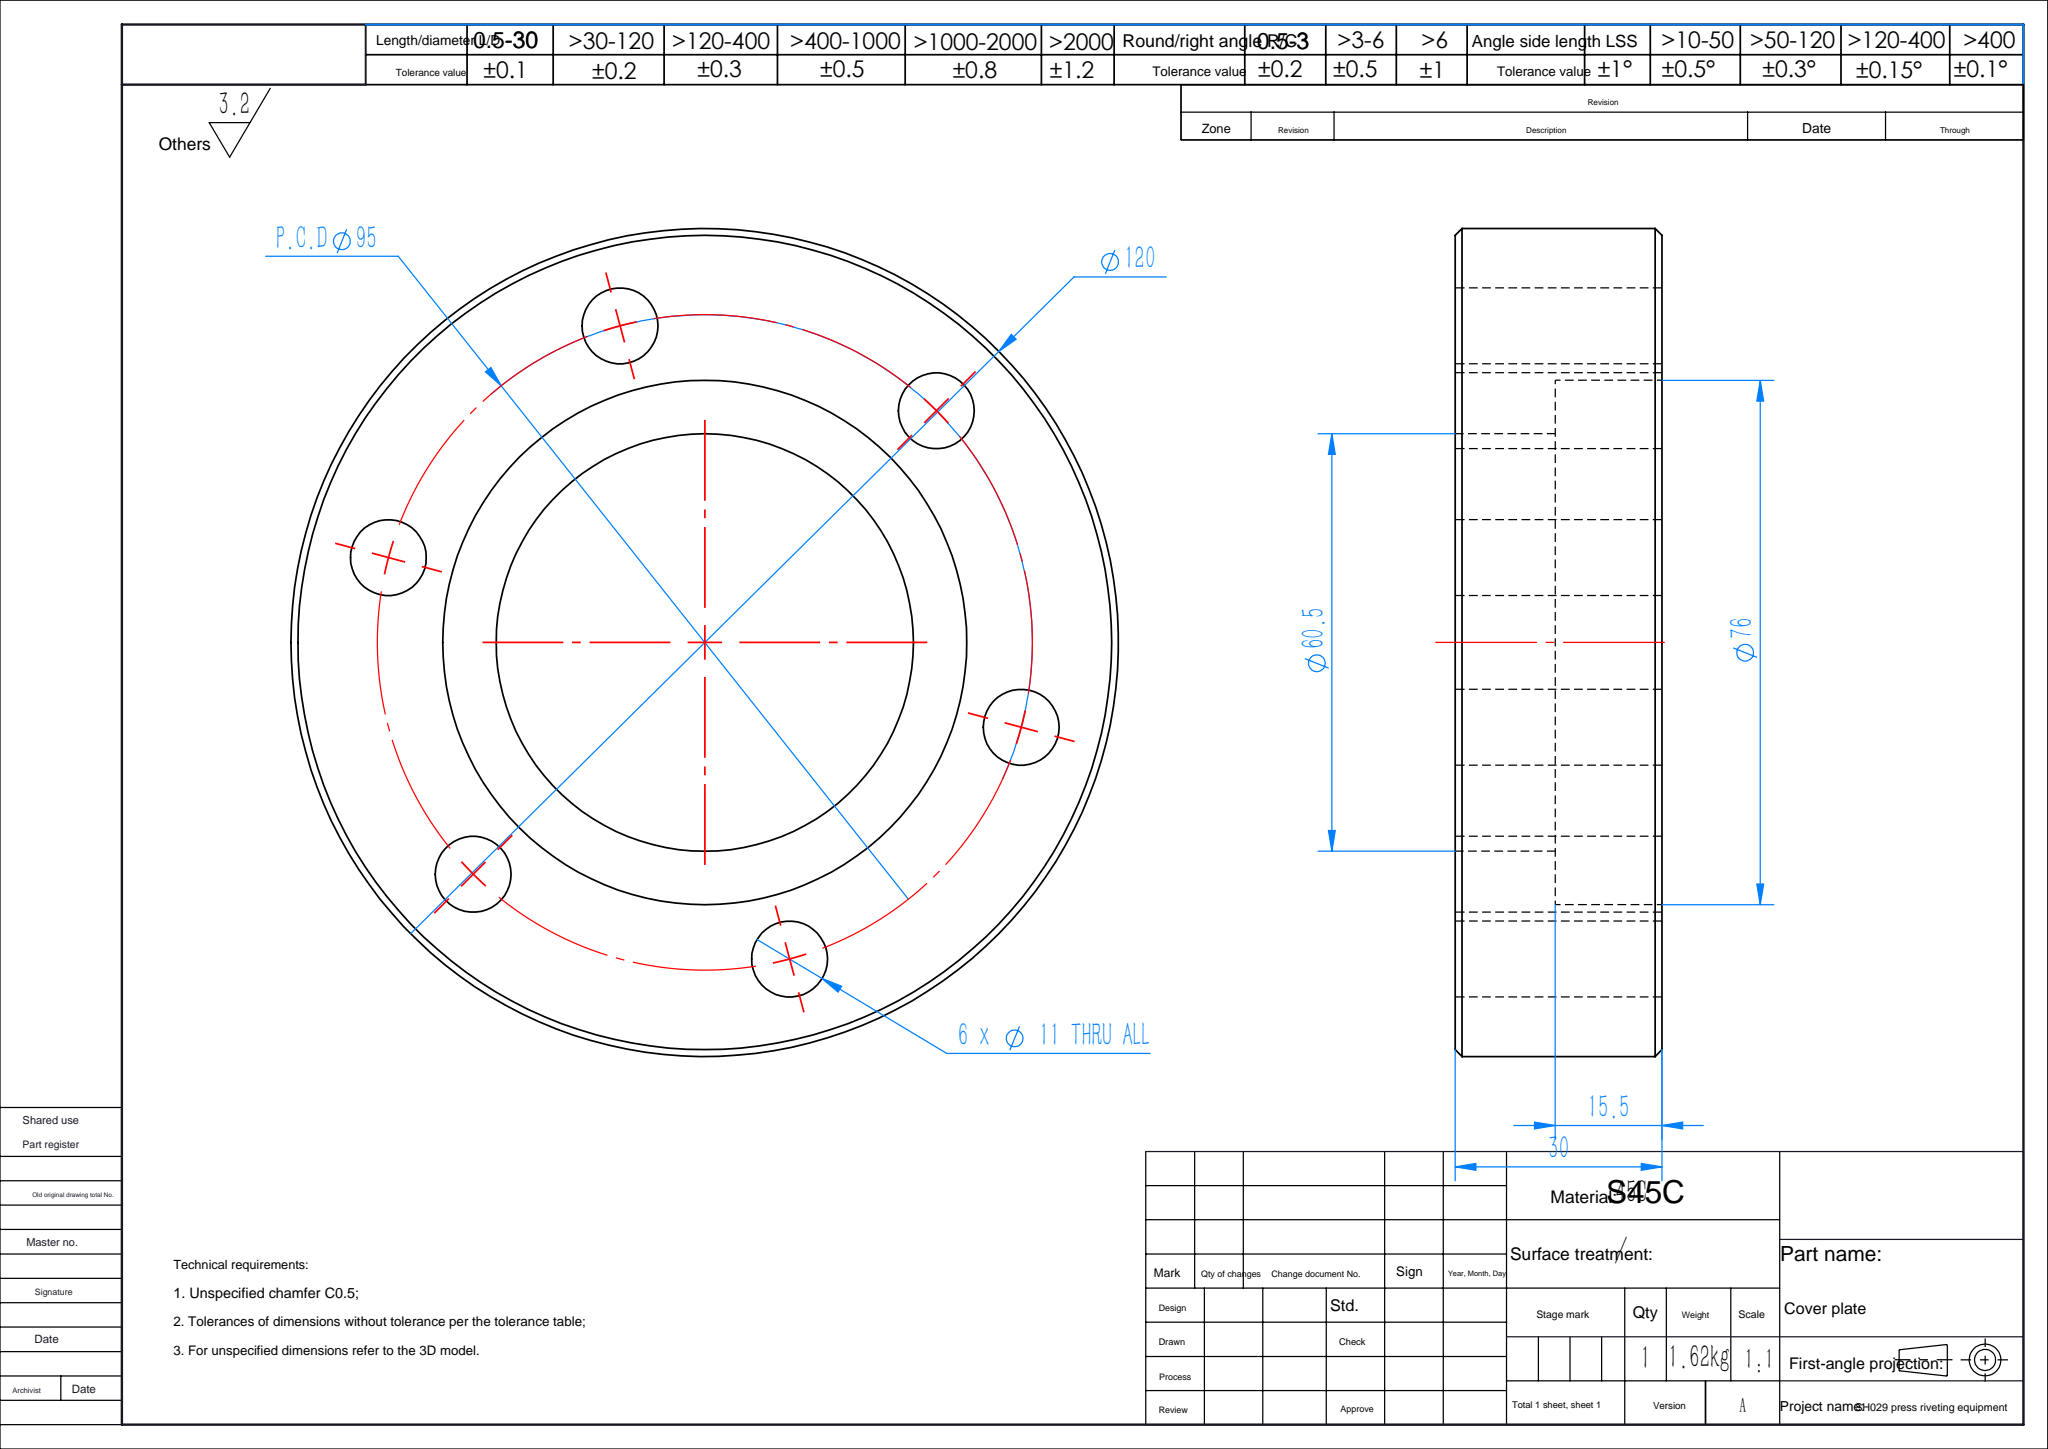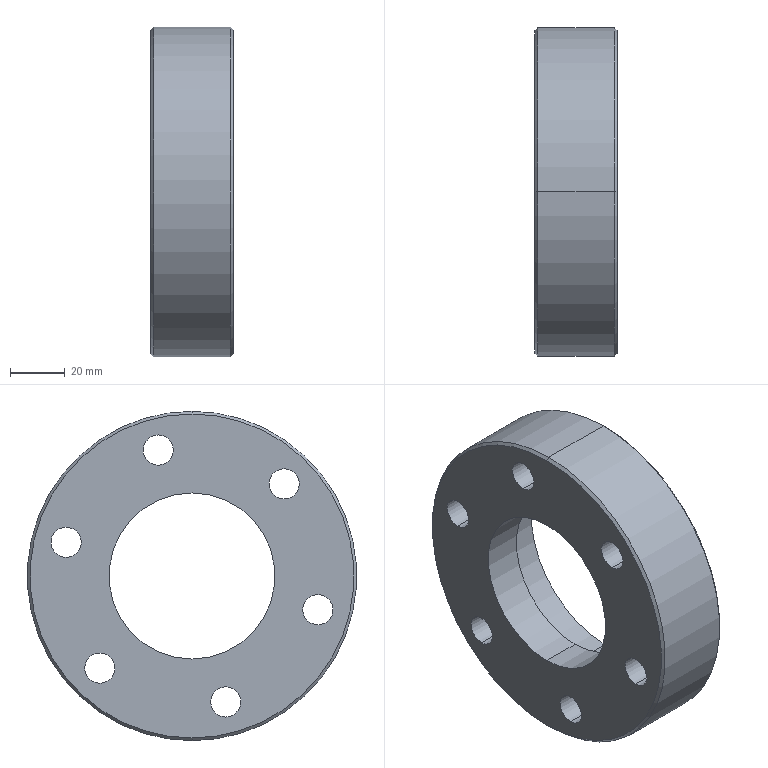Part | SolidWorks | features Chamfer 1, CirPattern 1, HoleWzd 1, Revolution 1 | 1 solid | 25 faces | box 30 x 120 x 120 mm | volume 209812 mm3 | cylinder 18 | cone 4 | plane 3 | commonest cylinder face diameters 11 x12 60.5 x2 76 x2 120 x2
STEP:
#1=CARTESIAN_POINT('',(15.,12.294,40.381));
#2=VERTEX_POINT('',#1);
#3=CARTESIAN_POINT('',(15.,12.294,51.381));
#4=VERTEX_POINT('',#3);
#5=CARTESIAN_POINT('',(15.,12.294,45.881));
#6=DIRECTION('',(-1.,0.,0.));
#7=DIRECTION('',(0.,0.,1.));
#8=AXIS2_PLACEMENT_3D('',#5,#6,#7);
#9=CIRCLE('',#8,5.5);
#10=EDGE_CURVE('',#2,#4,#9,.T.);
#11=ORIENTED_EDGE('',*,*,#10,.F.);
#12=CARTESIAN_POINT('',(-15.,12.294,40.381));
#13=VERTEX_POINT('',#12);
#14=CARTESIAN_POINT('',(-15.,12.294,40.381));
#15=DIRECTION('',(-1.,0.,0.));
#16=VECTOR('',#15,1000.);
#17=LINE('',#14,#16);
#18=EDGE_CURVE('',#2,#13,#17,.T.);
#19=ORIENTED_EDGE('',*,*,#18,.T.);
#20=CARTESIAN_POINT('',(-15.,12.294,51.381));
#21=VERTEX_POINT('',#20);
#22=CARTESIAN_POINT('',(-15.,12.294,45.881));
#23=DIRECTION('',(-1.,0.,0.));
#24=DIRECTION('',(0.,0.,1.));
#25=AXIS2_PLACEMENT_3D('',#22,#23,#24);
#26=CIRCLE('',#25,5.5);
#27=EDGE_CURVE('',#13,#21,#26,.T.);
#28=ORIENTED_EDGE('',*,*,#27,.T.);
#29=CARTESIAN_POINT('',(-15.,12.294,51.381));
#30=DIRECTION('',(-1.,0.,0.));
#31=VECTOR('',#30,1000.);
#32=LINE('',#29,#31);
#33=EDGE_CURVE('',#4,#21,#32,.T.);
#34=ORIENTED_EDGE('',*,*,#33,.F.);
#35=EDGE_LOOP('',(#11,#19,#28,#34));
#36=FACE_OUTER_BOUND('',#35,.T.);
#37=CARTESIAN_POINT('',(-15.,12.294,45.881));
#38=DIRECTION('',(-1.,0.,0.));
#39=DIRECTION('',(0.,0.,1.));
#40=AXIS2_PLACEMENT_3D('',#37,#38,#39);
#41=CYLINDRICAL_SURFACE('',#40,5.5);
#42=ADVANCED_FACE('',(#36),#41,.F.);
#43=CARTESIAN_POINT('',(15.,45.881,6.794));
#44=VERTEX_POINT('',#43);
#45=CARTESIAN_POINT('',(15.,45.881,17.794));
#46=VERTEX_POINT('',#45);
#47=CARTESIAN_POINT('',(15.,45.881,12.294));
#48=DIRECTION('',(-1.,0.,0.));
#49=DIRECTION('',(0.,0.,1.));
#50=AXIS2_PLACEMENT_3D('',#47,#48,#49);
#51=CIRCLE('',#50,5.5);
#52=EDGE_CURVE('',#44,#46,#51,.T.);
#53=ORIENTED_EDGE('',*,*,#52,.F.);
#54=CARTESIAN_POINT('',(-15.,45.881,6.794));
#55=VERTEX_POINT('',#54);
#56=CARTESIAN_POINT('',(-15.,45.881,6.794));
#57=DIRECTION('',(-1.,0.,0.));
#58=VECTOR('',#57,1000.);
#59=LINE('',#56,#58);
#60=EDGE_CURVE('',#44,#55,#59,.T.);
#61=ORIENTED_EDGE('',*,*,#60,.T.);
#62=CARTESIAN_POINT('',(-15.,45.881,17.794));
#63=VERTEX_POINT('',#62);
#64=CARTESIAN_POINT('',(-15.,45.881,12.294));
#65=DIRECTION('',(-1.,0.,0.));
#66=DIRECTION('',(0.,0.,1.));
#67=AXIS2_PLACEMENT_3D('',#64,#65,#66);
#68=CIRCLE('',#67,5.5);
#69=EDGE_CURVE('',#55,#63,#68,.T.);
#70=ORIENTED_EDGE('',*,*,#69,.T.);
#71=CARTESIAN_POINT('',(-15.,45.881,17.794));
#72=DIRECTION('',(-1.,0.,0.));
#73=VECTOR('',#72,1000.);
#74=LINE('',#71,#73);
#75=EDGE_CURVE('',#46,#63,#74,.T.);
#76=ORIENTED_EDGE('',*,*,#75,.F.);
#77=EDGE_LOOP('',(#53,#61,#70,#76));
#78=FACE_OUTER_BOUND('',#77,.T.);
#79=CARTESIAN_POINT('',(-15.,45.881,12.294));
#80=DIRECTION('',(-1.,0.,0.));
#81=DIRECTION('',(0.,0.,1.));
#82=AXIS2_PLACEMENT_3D('',#79,#80,#81);
#83=CYLINDRICAL_SURFACE('',#82,5.5);
#84=ADVANCED_FACE('',(#78),#83,.F.);
#85=CARTESIAN_POINT('',(15.,33.588,-39.088));
#86=VERTEX_POINT('',#85);
#87=CARTESIAN_POINT('',(15.,33.588,-28.088));
#88=VERTEX_POINT('',#87);
#89=CARTESIAN_POINT('',(15.,33.588,-33.588));
#90=DIRECTION('',(-1.,0.,0.));
#91=DIRECTION('',(0.,0.,1.));
#92=AXIS2_PLACEMENT_3D('',#89,#90,#91);
#93=CIRCLE('',#92,5.5);
#94=EDGE_CURVE('',#86,#88,#93,.T.);
#95=ORIENTED_EDGE('',*,*,#94,.F.);
#96=CARTESIAN_POINT('',(-15.,33.588,-39.088));
#97=VERTEX_POINT('',#96);
#98=CARTESIAN_POINT('',(-15.,33.588,-39.088));
#99=DIRECTION('',(-1.,0.,0.));
#100=VECTOR('',#99,1000.);
#101=LINE('',#98,#100);
#102=EDGE_CURVE('',#86,#97,#101,.T.);
#103=ORIENTED_EDGE('',*,*,#102,.T.);
#104=CARTESIAN_POINT('',(-15.,33.588,-28.088));
#105=VERTEX_POINT('',#104);
#106=CARTESIAN_POINT('',(-15.,33.588,-33.588));
#107=DIRECTION('',(-1.,0.,0.));
#108=DIRECTION('',(0.,0.,1.));
#109=AXIS2_PLACEMENT_3D('',#106,#107,#108);
#110=CIRCLE('',#109,5.5);
#111=EDGE_CURVE('',#97,#105,#110,.T.);
#112=ORIENTED_EDGE('',*,*,#111,.T.);
#113=CARTESIAN_POINT('',(-15.,33.588,-28.088));
#114=DIRECTION('',(-1.,0.,0.));
#115=VECTOR('',#114,1000.);
#116=LINE('',#113,#115);
#117=EDGE_CURVE('',#88,#105,#116,.T.);
#118=ORIENTED_EDGE('',*,*,#117,.F.);
#119=EDGE_LOOP('',(#95,#103,#112,#118));
#120=FACE_OUTER_BOUND('',#119,.T.);
#121=CARTESIAN_POINT('',(-15.,33.588,-33.588));
#122=DIRECTION('',(-1.,0.,0.));
#123=DIRECTION('',(0.,0.,1.));
#124=AXIS2_PLACEMENT_3D('',#121,#122,#123);
#125=CYLINDRICAL_SURFACE('',#124,5.5);
#126=ADVANCED_FACE('',(#120),#125,.F.);
#127=CARTESIAN_POINT('',(15.,-12.294,-51.381));
#128=VERTEX_POINT('',#127);
#129=CARTESIAN_POINT('',(15.,-12.294,-40.381));
#130=VERTEX_POINT('',#129);
#131=CARTESIAN_POINT('',(15.,-12.294,-45.881));
#132=DIRECTION('',(-1.,0.,0.));
#133=DIRECTION('',(0.,0.,1.));
#134=AXIS2_PLACEMENT_3D('',#131,#132,#133);
#135=CIRCLE('',#134,5.5);
#136=EDGE_CURVE('',#128,#130,#135,.T.);
#137=ORIENTED_EDGE('',*,*,#136,.F.);
#138=CARTESIAN_POINT('',(-15.,-12.294,-51.381));
#139=VERTEX_POINT('',#138);
#140=CARTESIAN_POINT('',(-15.,-12.294,-51.381));
#141=DIRECTION('',(-1.,0.,0.));
#142=VECTOR('',#141,1000.);
#143=LINE('',#140,#142);
#144=EDGE_CURVE('',#128,#139,#143,.T.);
#145=ORIENTED_EDGE('',*,*,#144,.T.);
#146=CARTESIAN_POINT('',(-15.,-12.294,-40.381));
#147=VERTEX_POINT('',#146);
#148=CARTESIAN_POINT('',(-15.,-12.294,-45.881));
#149=DIRECTION('',(-1.,0.,0.));
#150=DIRECTION('',(0.,0.,1.));
#151=AXIS2_PLACEMENT_3D('',#148,#149,#150);
#152=CIRCLE('',#151,5.5);
#153=EDGE_CURVE('',#139,#147,#152,.T.);
#154=ORIENTED_EDGE('',*,*,#153,.T.);
#155=CARTESIAN_POINT('',(-15.,-12.294,-40.381));
#156=DIRECTION('',(-1.,0.,0.));
#157=VECTOR('',#156,1000.);
#158=LINE('',#155,#157);
#159=EDGE_CURVE('',#130,#147,#158,.T.);
#160=ORIENTED_EDGE('',*,*,#159,.F.);
#161=EDGE_LOOP('',(#137,#145,#154,#160));
#162=FACE_OUTER_BOUND('',#161,.T.);
#163=CARTESIAN_POINT('',(-15.,-12.294,-45.881));
#164=DIRECTION('',(-1.,0.,0.));
#165=DIRECTION('',(0.,0.,1.));
#166=AXIS2_PLACEMENT_3D('',#163,#164,#165);
#167=CYLINDRICAL_SURFACE('',#166,5.5);
#168=ADVANCED_FACE('',(#162),#167,.F.);
#169=CARTESIAN_POINT('',(15.,-45.881,-17.794));
#170=VERTEX_POINT('',#169);
#171=CARTESIAN_POINT('',(15.,-45.881,-6.794));
#172=VERTEX_POINT('',#171);
#173=CARTESIAN_POINT('',(15.,-45.881,-12.294));
#174=DIRECTION('',(-1.,0.,0.));
#175=DIRECTION('',(0.,0.,1.));
#176=AXIS2_PLACEMENT_3D('',#173,#174,#175);
#177=CIRCLE('',#176,5.5);
#178=EDGE_CURVE('',#170,#172,#177,.T.);
#179=ORIENTED_EDGE('',*,*,#178,.F.);
#180=CARTESIAN_POINT('',(-15.,-45.881,-17.794));
#181=VERTEX_POINT('',#180);
#182=CARTESIAN_POINT('',(-15.,-45.881,-17.794));
#183=DIRECTION('',(-1.,0.,0.));
#184=VECTOR('',#183,1000.);
#185=LINE('',#182,#184);
#186=EDGE_CURVE('',#170,#181,#185,.T.);
#187=ORIENTED_EDGE('',*,*,#186,.T.);
#188=CARTESIAN_POINT('',(-15.,-45.881,-6.794));
#189=VERTEX_POINT('',#188);
#190=CARTESIAN_POINT('',(-15.,-45.881,-12.294));
#191=DIRECTION('',(-1.,0.,0.));
#192=DIRECTION('',(0.,0.,1.));
#193=AXIS2_PLACEMENT_3D('',#190,#191,#192);
#194=CIRCLE('',#193,5.5);
#195=EDGE_CURVE('',#181,#189,#194,.T.);
#196=ORIENTED_EDGE('',*,*,#195,.T.);
#197=CARTESIAN_POINT('',(-15.,-45.881,-6.794));
#198=DIRECTION('',(-1.,0.,0.));
#199=VECTOR('',#198,1000.);
#200=LINE('',#197,#199);
#201=EDGE_CURVE('',#172,#189,#200,.T.);
#202=ORIENTED_EDGE('',*,*,#201,.F.);
#203=EDGE_LOOP('',(#179,#187,#196,#202));
#204=FACE_OUTER_BOUND('',#203,.T.);
#205=CARTESIAN_POINT('',(-15.,-45.881,-12.294));
#206=DIRECTION('',(-1.,0.,0.));
#207=DIRECTION('',(0.,0.,1.));
#208=AXIS2_PLACEMENT_3D('',#205,#206,#207);
#209=CYLINDRICAL_SURFACE('',#208,5.5);
#210=ADVANCED_FACE('',(#204),#209,.F.);
#211=CARTESIAN_POINT('',(15.,-33.588,28.088));
#212=VERTEX_POINT('',#211);
#213=CARTESIAN_POINT('',(15.,-33.588,39.088));
#214=VERTEX_POINT('',#213);
#215=CARTESIAN_POINT('',(15.,-33.588,33.588));
#216=DIRECTION('',(-1.,0.,0.));
#217=DIRECTION('',(0.,0.,1.));
#218=AXIS2_PLACEMENT_3D('',#215,#216,#217);
#219=CIRCLE('',#218,5.5);
#220=EDGE_CURVE('',#212,#214,#219,.T.);
#221=ORIENTED_EDGE('',*,*,#220,.F.);
#222=CARTESIAN_POINT('',(-15.,-33.588,28.088));
#223=VERTEX_POINT('',#222);
#224=CARTESIAN_POINT('',(-15.,-33.588,28.088));
#225=DIRECTION('',(-1.,0.,0.));
#226=VECTOR('',#225,1000.);
#227=LINE('',#224,#226);
#228=EDGE_CURVE('',#212,#223,#227,.T.);
#229=ORIENTED_EDGE('',*,*,#228,.T.);
#230=CARTESIAN_POINT('',(-15.,-33.588,39.088));
#231=VERTEX_POINT('',#230);
#232=CARTESIAN_POINT('',(-15.,-33.588,33.588));
#233=DIRECTION('',(-1.,0.,0.));
#234=DIRECTION('',(0.,0.,1.));
#235=AXIS2_PLACEMENT_3D('',#232,#233,#234);
#236=CIRCLE('',#235,5.5);
#237=EDGE_CURVE('',#223,#231,#236,.T.);
#238=ORIENTED_EDGE('',*,*,#237,.T.);
#239=CARTESIAN_POINT('',(-15.,-33.588,39.088));
#240=DIRECTION('',(-1.,0.,0.));
#241=VECTOR('',#240,1000.);
#242=LINE('',#239,#241);
#243=EDGE_CURVE('',#214,#231,#242,.T.);
#244=ORIENTED_EDGE('',*,*,#243,.F.);
#245=EDGE_LOOP('',(#221,#229,#238,#244));
#246=FACE_OUTER_BOUND('',#245,.T.);
#247=CARTESIAN_POINT('',(-15.,-33.588,33.588));
#248=DIRECTION('',(-1.,0.,0.));
#249=DIRECTION('',(0.,0.,1.));
#250=AXIS2_PLACEMENT_3D('',#247,#248,#249);
#251=CYLINDRICAL_SURFACE('',#250,5.5);
#252=ADVANCED_FACE('',(#246),#251,.F.);
#253=CARTESIAN_POINT('',(-15.,0.,59.));
#254=VERTEX_POINT('',#253);
#255=CARTESIAN_POINT('',(-15.,0.,-59.));
#256=VERTEX_POINT('',#255);
#257=CARTESIAN_POINT('',(-15.,0.,0.));
#258=DIRECTION('',(-1.,0.,0.));
#259=DIRECTION('',(0.,0.,-1.));
#260=AXIS2_PLACEMENT_3D('',#257,#258,#259);
#261=CIRCLE('',#260,59.);
#262=EDGE_CURVE('',#254,#256,#261,.T.);
#263=ORIENTED_EDGE('',*,*,#262,.F.);
#264=CARTESIAN_POINT('',(-14.,0.,60.));
#265=VERTEX_POINT('',#264);
#266=CARTESIAN_POINT('',(-15.,0.,59.));
#267=DIRECTION('',(0.7071,0.,0.7071));
#268=VECTOR('',#267,1000.);
#269=LINE('',#266,#268);
#270=EDGE_CURVE('',#254,#265,#269,.T.);
#271=ORIENTED_EDGE('',*,*,#270,.T.);
#272=CARTESIAN_POINT('',(-14.,0.,-60.));
#273=VERTEX_POINT('',#272);
#274=CARTESIAN_POINT('',(-14.,0.,0.));
#275=DIRECTION('',(1.,0.,0.));
#276=DIRECTION('',(0.,0.,-1.));
#277=AXIS2_PLACEMENT_3D('',#274,#275,#276);
#278=CIRCLE('',#277,60.);
#279=EDGE_CURVE('',#273,#265,#278,.T.);
#280=ORIENTED_EDGE('',*,*,#279,.F.);
#281=CARTESIAN_POINT('',(-15.,0.,-59.));
#282=DIRECTION('',(0.7071,0.,-0.7071));
#283=VECTOR('',#282,1000.);
#284=LINE('',#281,#283);
#285=EDGE_CURVE('',#256,#273,#284,.T.);
#286=ORIENTED_EDGE('',*,*,#285,.F.);
#287=EDGE_LOOP('',(#263,#271,#280,#286));
#288=FACE_OUTER_BOUND('',#287,.T.);
#289=CARTESIAN_POINT('',(-15.,0.,0.));
#290=DIRECTION('',(1.,0.,0.));
#291=DIRECTION('',(0.,0.,-1.));
#292=AXIS2_PLACEMENT_3D('',#289,#290,#291);
#293=CONICAL_SURFACE('',#292,59.,0.7854);
#294=ADVANCED_FACE('',(#288),#293,.T.);
#295=CARTESIAN_POINT('',(15.,0.,-59.));
#296=VERTEX_POINT('',#295);
#297=CARTESIAN_POINT('',(15.,0.,59.));
#298=VERTEX_POINT('',#297);
#299=CARTESIAN_POINT('',(15.,0.,0.));
#300=DIRECTION('',(1.,0.,0.));
#301=DIRECTION('',(0.,0.,1.));
#302=AXIS2_PLACEMENT_3D('',#299,#300,#301);
#303=CIRCLE('',#302,59.);
#304=EDGE_CURVE('',#296,#298,#303,.T.);
#305=ORIENTED_EDGE('',*,*,#304,.F.);
#306=CARTESIAN_POINT('',(14.,0.,-60.));
#307=VERTEX_POINT('',#306);
#308=CARTESIAN_POINT('',(14.,0.,-60.));
#309=DIRECTION('',(-0.7071,0.,-0.7071));
#310=VECTOR('',#309,1000.);
#311=LINE('',#308,#310);
#312=EDGE_CURVE('',#296,#307,#311,.T.);
#313=ORIENTED_EDGE('',*,*,#312,.T.);
#314=CARTESIAN_POINT('',(14.,0.,60.));
#315=VERTEX_POINT('',#314);
#316=CARTESIAN_POINT('',(14.,0.,0.));
#317=DIRECTION('',(-1.,0.,0.));
#318=DIRECTION('',(0.,0.,1.));
#319=AXIS2_PLACEMENT_3D('',#316,#317,#318);
#320=CIRCLE('',#319,60.);
#321=EDGE_CURVE('',#315,#307,#320,.T.);
#322=ORIENTED_EDGE('',*,*,#321,.F.);
#323=CARTESIAN_POINT('',(14.,0.,60.));
#324=DIRECTION('',(-0.7071,0.,0.7071));
#325=VECTOR('',#324,1000.);
#326=LINE('',#323,#325);
#327=EDGE_CURVE('',#298,#315,#326,.T.);
#328=ORIENTED_EDGE('',*,*,#327,.F.);
#329=EDGE_LOOP('',(#305,#313,#322,#328));
#330=FACE_OUTER_BOUND('',#329,.T.);
#331=CARTESIAN_POINT('',(14.,0.,0.));
#332=DIRECTION('',(-1.,0.,0.));
#333=DIRECTION('',(0.,0.,1.));
#334=AXIS2_PLACEMENT_3D('',#331,#332,#333);
#335=CONICAL_SURFACE('',#334,60.,0.7854);
#336=ADVANCED_FACE('',(#330),#335,.T.);
#337=CARTESIAN_POINT('',(-0.5,0.,-30.25));
#338=VERTEX_POINT('',#337);
#339=CARTESIAN_POINT('',(-0.5,0.,30.25));
#340=VERTEX_POINT('',#339);
#341=CARTESIAN_POINT('',(-0.5,0.,0.));
#342=DIRECTION('',(-1.,0.,0.));
#343=DIRECTION('',(0.,0.,1.));
#344=AXIS2_PLACEMENT_3D('',#341,#342,#343);
#345=CIRCLE('',#344,30.25);
#346=EDGE_CURVE('',#338,#340,#345,.T.);
#347=ORIENTED_EDGE('',*,*,#346,.F.);
#348=CARTESIAN_POINT('',(-15.,0.,-30.25));
#349=VERTEX_POINT('',#348);
#350=CARTESIAN_POINT('',(-222.715,0.,-30.25));
#351=DIRECTION('',(-1.,0.,0.));
#352=VECTOR('',#351,1000.);
#353=LINE('',#350,#352);
#354=EDGE_CURVE('',#338,#349,#353,.T.);
#355=ORIENTED_EDGE('',*,*,#354,.T.);
#356=CARTESIAN_POINT('',(-15.,0.,30.25));
#357=VERTEX_POINT('',#356);
#358=CARTESIAN_POINT('',(-15.,0.,0.));
#359=DIRECTION('',(-1.,0.,0.));
#360=DIRECTION('',(0.,0.,1.));
#361=AXIS2_PLACEMENT_3D('',#358,#359,#360);
#362=CIRCLE('',#361,30.25);
#363=EDGE_CURVE('',#349,#357,#362,.T.);
#364=ORIENTED_EDGE('',*,*,#363,.T.);
#365=CARTESIAN_POINT('',(-222.715,0.,30.25));
#366=DIRECTION('',(-1.,0.,0.));
#367=VECTOR('',#366,1000.);
#368=LINE('',#365,#367);
#369=EDGE_CURVE('',#340,#357,#368,.T.);
#370=ORIENTED_EDGE('',*,*,#369,.F.);
#371=EDGE_LOOP('',(#347,#355,#364,#370));
#372=FACE_OUTER_BOUND('',#371,.T.);
#373=CARTESIAN_POINT('',(-222.715,0.,0.));
#374=DIRECTION('',(-1.,0.,0.));
#375=DIRECTION('',(0.,0.,1.));
#376=AXIS2_PLACEMENT_3D('',#373,#374,#375);
#377=CYLINDRICAL_SURFACE('',#376,30.25);
#378=ADVANCED_FACE('',(#372),#377,.F.);
#379=CARTESIAN_POINT('',(15.,0.,-38.));
#380=VERTEX_POINT('',#379);
#381=CARTESIAN_POINT('',(15.,0.,38.));
#382=VERTEX_POINT('',#381);
#383=CARTESIAN_POINT('',(15.,0.,0.));
#384=DIRECTION('',(-1.,0.,0.));
#385=DIRECTION('',(0.,0.,1.));
#386=AXIS2_PLACEMENT_3D('',#383,#384,#385);
#387=CIRCLE('',#386,38.);
#388=EDGE_CURVE('',#380,#382,#387,.T.);
#389=ORIENTED_EDGE('',*,*,#388,.F.);
#390=CARTESIAN_POINT('',(-0.5,0.,-38.));
#391=VERTEX_POINT('',#390);
#392=CARTESIAN_POINT('',(-222.715,0.,-38.));
#393=DIRECTION('',(-1.,0.,0.));
#394=VECTOR('',#393,1000.);
#395=LINE('',#392,#394);
#396=EDGE_CURVE('',#380,#391,#395,.T.);
#397=ORIENTED_EDGE('',*,*,#396,.T.);
#398=CARTESIAN_POINT('',(-0.5,0.,38.));
#399=VERTEX_POINT('',#398);
#400=CARTESIAN_POINT('',(-0.5,0.,0.));
#401=DIRECTION('',(-1.,0.,0.));
#402=DIRECTION('',(0.,0.,1.));
#403=AXIS2_PLACEMENT_3D('',#400,#401,#402);
#404=CIRCLE('',#403,38.);
#405=EDGE_CURVE('',#391,#399,#404,.T.);
#406=ORIENTED_EDGE('',*,*,#405,.T.);
#407=CARTESIAN_POINT('',(-222.715,0.,38.));
#408=DIRECTION('',(-1.,0.,0.));
#409=VECTOR('',#408,1000.);
#410=LINE('',#407,#409);
#411=EDGE_CURVE('',#382,#399,#410,.T.);
#412=ORIENTED_EDGE('',*,*,#411,.F.);
#413=EDGE_LOOP('',(#389,#397,#406,#412));
#414=FACE_OUTER_BOUND('',#413,.T.);
#415=CARTESIAN_POINT('',(-222.715,0.,0.));
#416=DIRECTION('',(-1.,0.,0.));
#417=DIRECTION('',(0.,0.,1.));
#418=AXIS2_PLACEMENT_3D('',#415,#416,#417);
#419=CYLINDRICAL_SURFACE('',#418,38.);
#420=ADVANCED_FACE('',(#414),#419,.F.);
#421=ORIENTED_EDGE('',*,*,#321,.T.);
#422=CARTESIAN_POINT('',(-222.715,0.,-60.));
#423=DIRECTION('',(-1.,0.,0.));
#424=VECTOR('',#423,1000.);
#425=LINE('',#422,#424);
#426=EDGE_CURVE('',#307,#273,#425,.T.);
#427=ORIENTED_EDGE('',*,*,#426,.T.);
#428=ORIENTED_EDGE('',*,*,#279,.T.);
#429=CARTESIAN_POINT('',(-222.715,0.,60.));
#430=DIRECTION('',(-1.,0.,0.));
#431=VECTOR('',#430,1000.);
#432=LINE('',#429,#431);
#433=EDGE_CURVE('',#315,#265,#432,.T.);
#434=ORIENTED_EDGE('',*,*,#433,.F.);
#435=EDGE_LOOP('',(#421,#427,#428,#434));
#436=FACE_OUTER_BOUND('',#435,.T.);
#437=CARTESIAN_POINT('',(-222.715,0.,0.));
#438=DIRECTION('',(-1.,0.,0.));
#439=DIRECTION('',(0.,0.,1.));
#440=AXIS2_PLACEMENT_3D('',#437,#438,#439);
#441=CYLINDRICAL_SURFACE('',#440,60.);
#442=ADVANCED_FACE('',(#436),#441,.T.);
#443=CARTESIAN_POINT('',(-15.,12.294,45.881));
#444=DIRECTION('',(-1.,0.,0.));
#445=DIRECTION('',(0.,0.,1.));
#446=AXIS2_PLACEMENT_3D('',#443,#444,#445);
#447=CIRCLE('',#446,5.5);
#448=EDGE_CURVE('',#21,#13,#447,.T.);
#449=ORIENTED_EDGE('',*,*,#448,.F.);
#450=ORIENTED_EDGE('',*,*,#27,.F.);
#451=EDGE_LOOP('',(#449,#450));
#452=FACE_BOUND('',#451,.T.);
#453=CARTESIAN_POINT('',(-15.,45.881,12.294));
#454=DIRECTION('',(-1.,0.,0.));
#455=DIRECTION('',(0.,0.,1.));
#456=AXIS2_PLACEMENT_3D('',#453,#454,#455);
#457=CIRCLE('',#456,5.5);
#458=EDGE_CURVE('',#63,#55,#457,.T.);
#459=ORIENTED_EDGE('',*,*,#458,.F.);
#460=ORIENTED_EDGE('',*,*,#69,.F.);
#461=EDGE_LOOP('',(#459,#460));
#462=FACE_BOUND('',#461,.T.);
#463=CARTESIAN_POINT('',(-15.,-12.294,-45.881));
#464=DIRECTION('',(-1.,0.,0.));
#465=DIRECTION('',(0.,0.,1.));
#466=AXIS2_PLACEMENT_3D('',#463,#464,#465);
#467=CIRCLE('',#466,5.5);
#468=EDGE_CURVE('',#147,#139,#467,.T.);
#469=ORIENTED_EDGE('',*,*,#468,.F.);
#470=ORIENTED_EDGE('',*,*,#153,.F.);
#471=EDGE_LOOP('',(#469,#470));
#472=FACE_BOUND('',#471,.T.);
#473=CARTESIAN_POINT('',(-15.,-33.588,33.588));
#474=DIRECTION('',(-1.,0.,0.));
#475=DIRECTION('',(0.,0.,1.));
#476=AXIS2_PLACEMENT_3D('',#473,#474,#475);
#477=CIRCLE('',#476,5.5);
#478=EDGE_CURVE('',#231,#223,#477,.T.);
#479=ORIENTED_EDGE('',*,*,#478,.F.);
#480=ORIENTED_EDGE('',*,*,#237,.F.);
#481=EDGE_LOOP('',(#479,#480));
#482=FACE_BOUND('',#481,.T.);
#483=CARTESIAN_POINT('',(-15.,0.,0.));
#484=DIRECTION('',(-1.,0.,0.));
#485=DIRECTION('',(0.,0.,-1.));
#486=AXIS2_PLACEMENT_3D('',#483,#484,#485);
#487=CIRCLE('',#486,59.);
#488=EDGE_CURVE('',#256,#254,#487,.T.);
#489=ORIENTED_EDGE('',*,*,#488,.T.);
#490=ORIENTED_EDGE('',*,*,#262,.T.);
#491=EDGE_LOOP('',(#489,#490));
#492=FACE_OUTER_BOUND('',#491,.T.);
#493=CARTESIAN_POINT('',(-15.,0.,0.));
#494=DIRECTION('',(-1.,0.,0.));
#495=DIRECTION('',(0.,0.,1.));
#496=AXIS2_PLACEMENT_3D('',#493,#494,#495);
#497=CIRCLE('',#496,30.25);
#498=EDGE_CURVE('',#357,#349,#497,.T.);
#499=ORIENTED_EDGE('',*,*,#498,.F.);
#500=ORIENTED_EDGE('',*,*,#363,.F.);
#501=EDGE_LOOP('',(#499,#500));
#502=FACE_BOUND('',#501,.T.);
#503=CARTESIAN_POINT('',(-15.,-45.881,-12.294));
#504=DIRECTION('',(-1.,0.,0.));
#505=DIRECTION('',(0.,0.,1.));
#506=AXIS2_PLACEMENT_3D('',#503,#504,#505);
#507=CIRCLE('',#506,5.5);
#508=EDGE_CURVE('',#189,#181,#507,.T.);
#509=ORIENTED_EDGE('',*,*,#508,.F.);
#510=ORIENTED_EDGE('',*,*,#195,.F.);
#511=EDGE_LOOP('',(#509,#510));
#512=FACE_BOUND('',#511,.T.);
#513=CARTESIAN_POINT('',(-15.,33.588,-33.588));
#514=DIRECTION('',(-1.,0.,0.));
#515=DIRECTION('',(0.,0.,1.));
#516=AXIS2_PLACEMENT_3D('',#513,#514,#515);
#517=CIRCLE('',#516,5.5);
#518=EDGE_CURVE('',#105,#97,#517,.T.);
#519=ORIENTED_EDGE('',*,*,#518,.F.);
#520=ORIENTED_EDGE('',*,*,#111,.F.);
#521=EDGE_LOOP('',(#519,#520));
#522=FACE_BOUND('',#521,.T.);
#523=CARTESIAN_POINT('',(-15.,0.,-30.25));
#524=DIRECTION('',(1.,0.,0.));
#525=DIRECTION('',(0.,0.,-1.));
#526=AXIS2_PLACEMENT_3D('',#523,#524,#525);
#527=PLANE('',#526);
#528=ADVANCED_FACE('',(#452,#462,#472,#482,#492,#502,#512,#522),#527,.F.);
#529=ORIENTED_EDGE('',*,*,#426,.F.);
#530=CARTESIAN_POINT('',(14.,0.,0.));
#531=DIRECTION('',(-1.,0.,0.));
#532=DIRECTION('',(0.,0.,1.));
#533=AXIS2_PLACEMENT_3D('',#530,#531,#532);
#534=CIRCLE('',#533,60.);
#535=EDGE_CURVE('',#307,#315,#534,.T.);
#536=ORIENTED_EDGE('',*,*,#535,.T.);
#537=ORIENTED_EDGE('',*,*,#433,.T.);
#538=CARTESIAN_POINT('',(-14.,0.,0.));
#539=DIRECTION('',(1.,0.,0.));
#540=DIRECTION('',(0.,0.,-1.));
#541=AXIS2_PLACEMENT_3D('',#538,#539,#540);
#542=CIRCLE('',#541,60.);
#543=EDGE_CURVE('',#265,#273,#542,.T.);
#544=ORIENTED_EDGE('',*,*,#543,.T.);
#545=EDGE_LOOP('',(#529,#536,#537,#544));
#546=FACE_OUTER_BOUND('',#545,.T.);
#547=CARTESIAN_POINT('',(-222.715,0.,0.));
#548=DIRECTION('',(-1.,0.,0.));
#549=DIRECTION('',(0.,0.,1.));
#550=AXIS2_PLACEMENT_3D('',#547,#548,#549);
#551=CYLINDRICAL_SURFACE('',#550,60.);
#552=ADVANCED_FACE('',(#546),#551,.T.);
#553=CARTESIAN_POINT('',(15.,12.294,45.881));
#554=DIRECTION('',(-1.,0.,0.));
#555=DIRECTION('',(0.,0.,1.));
#556=AXIS2_PLACEMENT_3D('',#553,#554,#555);
#557=CIRCLE('',#556,5.5);
#558=EDGE_CURVE('',#4,#2,#557,.T.);
#559=ORIENTED_EDGE('',*,*,#558,.T.);
#560=ORIENTED_EDGE('',*,*,#10,.T.);
#561=EDGE_LOOP('',(#559,#560));
#562=FACE_BOUND('',#561,.T.);
#563=CARTESIAN_POINT('',(15.,45.881,12.294));
#564=DIRECTION('',(-1.,0.,0.));
#565=DIRECTION('',(0.,0.,1.));
#566=AXIS2_PLACEMENT_3D('',#563,#564,#565);
#567=CIRCLE('',#566,5.5);
#568=EDGE_CURVE('',#46,#44,#567,.T.);
#569=ORIENTED_EDGE('',*,*,#568,.T.);
#570=ORIENTED_EDGE('',*,*,#52,.T.);
#571=EDGE_LOOP('',(#569,#570));
#572=FACE_BOUND('',#571,.T.);
#573=CARTESIAN_POINT('',(15.,33.588,-33.588));
#574=DIRECTION('',(-1.,0.,0.));
#575=DIRECTION('',(0.,0.,1.));
#576=AXIS2_PLACEMENT_3D('',#573,#574,#575);
#577=CIRCLE('',#576,5.5);
#578=EDGE_CURVE('',#88,#86,#577,.T.);
#579=ORIENTED_EDGE('',*,*,#578,.T.);
#580=ORIENTED_EDGE('',*,*,#94,.T.);
#581=EDGE_LOOP('',(#579,#580));
#582=FACE_BOUND('',#581,.T.);
#583=CARTESIAN_POINT('',(15.,-12.294,-45.881));
#584=DIRECTION('',(-1.,0.,0.));
#585=DIRECTION('',(0.,0.,1.));
#586=AXIS2_PLACEMENT_3D('',#583,#584,#585);
#587=CIRCLE('',#586,5.5);
#588=EDGE_CURVE('',#130,#128,#587,.T.);
#589=ORIENTED_EDGE('',*,*,#588,.T.);
#590=ORIENTED_EDGE('',*,*,#136,.T.);
#591=EDGE_LOOP('',(#589,#590));
#592=FACE_BOUND('',#591,.T.);
#593=CARTESIAN_POINT('',(15.,-45.881,-12.294));
#594=DIRECTION('',(-1.,0.,0.));
#595=DIRECTION('',(0.,0.,1.));
#596=AXIS2_PLACEMENT_3D('',#593,#594,#595);
#597=CIRCLE('',#596,5.5);
#598=EDGE_CURVE('',#172,#170,#597,.T.);
#599=ORIENTED_EDGE('',*,*,#598,.T.);
#600=ORIENTED_EDGE('',*,*,#178,.T.);
#601=EDGE_LOOP('',(#599,#600));
#602=FACE_BOUND('',#601,.T.);
#603=CARTESIAN_POINT('',(15.,-33.588,33.588));
#604=DIRECTION('',(-1.,0.,0.));
#605=DIRECTION('',(0.,0.,1.));
#606=AXIS2_PLACEMENT_3D('',#603,#604,#605);
#607=CIRCLE('',#606,5.5);
#608=EDGE_CURVE('',#214,#212,#607,.T.);
#609=ORIENTED_EDGE('',*,*,#608,.T.);
#610=ORIENTED_EDGE('',*,*,#220,.T.);
#611=EDGE_LOOP('',(#609,#610));
#612=FACE_BOUND('',#611,.T.);
#613=CARTESIAN_POINT('',(15.,0.,0.));
#614=DIRECTION('',(1.,0.,0.));
#615=DIRECTION('',(0.,0.,1.));
#616=AXIS2_PLACEMENT_3D('',#613,#614,#615);
#617=CIRCLE('',#616,59.);
#618=EDGE_CURVE('',#298,#296,#617,.T.);
#619=ORIENTED_EDGE('',*,*,#618,.T.);
#620=ORIENTED_EDGE('',*,*,#304,.T.);
#621=EDGE_LOOP('',(#619,#620));
#622=FACE_OUTER_BOUND('',#621,.T.);
#623=CARTESIAN_POINT('',(15.,0.,0.));
#624=DIRECTION('',(-1.,0.,0.));
#625=DIRECTION('',(0.,0.,1.));
#626=AXIS2_PLACEMENT_3D('',#623,#624,#625);
#627=CIRCLE('',#626,38.);
#628=EDGE_CURVE('',#382,#380,#627,.T.);
#629=ORIENTED_EDGE('',*,*,#628,.T.);
#630=ORIENTED_EDGE('',*,*,#388,.T.);
#631=EDGE_LOOP('',(#629,#630));
#632=FACE_BOUND('',#631,.T.);
#633=CARTESIAN_POINT('',(15.,0.,-60.));
#634=DIRECTION('',(-1.,0.,0.));
#635=DIRECTION('',(0.,0.,1.));
#636=AXIS2_PLACEMENT_3D('',#633,#634,#635);
#637=PLANE('',#636);
#638=ADVANCED_FACE('',(#562,#572,#582,#592,#602,#612,#622,#632),#637,.F.);
#639=ORIENTED_EDGE('',*,*,#396,.F.);
#640=ORIENTED_EDGE('',*,*,#628,.F.);
#641=ORIENTED_EDGE('',*,*,#411,.T.);
#642=CARTESIAN_POINT('',(-0.5,0.,0.));
#643=DIRECTION('',(-1.,0.,0.));
#644=DIRECTION('',(0.,0.,1.));
#645=AXIS2_PLACEMENT_3D('',#642,#643,#644);
#646=CIRCLE('',#645,38.);
#647=EDGE_CURVE('',#399,#391,#646,.T.);
#648=ORIENTED_EDGE('',*,*,#647,.T.);
#649=EDGE_LOOP('',(#639,#640,#641,#648));
#650=FACE_OUTER_BOUND('',#649,.T.);
#651=CARTESIAN_POINT('',(-222.715,0.,0.));
#652=DIRECTION('',(-1.,0.,0.));
#653=DIRECTION('',(0.,0.,1.));
#654=AXIS2_PLACEMENT_3D('',#651,#652,#653);
#655=CYLINDRICAL_SURFACE('',#654,38.);
#656=ADVANCED_FACE('',(#650),#655,.F.);
#657=ORIENTED_EDGE('',*,*,#647,.F.);
#658=ORIENTED_EDGE('',*,*,#405,.F.);
#659=EDGE_LOOP('',(#657,#658));
#660=FACE_OUTER_BOUND('',#659,.T.);
#661=CARTESIAN_POINT('',(-0.5,0.,0.));
#662=DIRECTION('',(-1.,0.,0.));
#663=DIRECTION('',(0.,0.,1.));
#664=AXIS2_PLACEMENT_3D('',#661,#662,#663);
#665=CIRCLE('',#664,30.25);
#666=EDGE_CURVE('',#340,#338,#665,.T.);
#667=ORIENTED_EDGE('',*,*,#666,.T.);
#668=ORIENTED_EDGE('',*,*,#346,.T.);
#669=EDGE_LOOP('',(#667,#668));
#670=FACE_BOUND('',#669,.T.);
#671=CARTESIAN_POINT('',(-0.5,0.,-38.));
#672=DIRECTION('',(-1.,0.,0.));
#673=DIRECTION('',(0.,0.,1.));
#674=AXIS2_PLACEMENT_3D('',#671,#672,#673);
#675=PLANE('',#674);
#676=ADVANCED_FACE('',(#660,#670),#675,.F.);
#677=ORIENTED_EDGE('',*,*,#354,.F.);
#678=ORIENTED_EDGE('',*,*,#666,.F.);
#679=ORIENTED_EDGE('',*,*,#369,.T.);
#680=ORIENTED_EDGE('',*,*,#498,.T.);
#681=EDGE_LOOP('',(#677,#678,#679,#680));
#682=FACE_OUTER_BOUND('',#681,.T.);
#683=CARTESIAN_POINT('',(-222.715,0.,0.));
#684=DIRECTION('',(-1.,0.,0.));
#685=DIRECTION('',(0.,0.,1.));
#686=AXIS2_PLACEMENT_3D('',#683,#684,#685);
#687=CYLINDRICAL_SURFACE('',#686,30.25);
#688=ADVANCED_FACE('',(#682),#687,.F.);
#689=ORIENTED_EDGE('',*,*,#312,.F.);
#690=ORIENTED_EDGE('',*,*,#618,.F.);
#691=ORIENTED_EDGE('',*,*,#327,.T.);
#692=ORIENTED_EDGE('',*,*,#535,.F.);
#693=EDGE_LOOP('',(#689,#690,#691,#692));
#694=FACE_OUTER_BOUND('',#693,.T.);
#695=CARTESIAN_POINT('',(14.,0.,0.));
#696=DIRECTION('',(-1.,0.,0.));
#697=DIRECTION('',(0.,0.,1.));
#698=AXIS2_PLACEMENT_3D('',#695,#696,#697);
#699=CONICAL_SURFACE('',#698,60.,0.7854);
#700=ADVANCED_FACE('',(#694),#699,.T.);
#701=ORIENTED_EDGE('',*,*,#270,.F.);
#702=ORIENTED_EDGE('',*,*,#488,.F.);
#703=ORIENTED_EDGE('',*,*,#285,.T.);
#704=ORIENTED_EDGE('',*,*,#543,.F.);
#705=EDGE_LOOP('',(#701,#702,#703,#704));
#706=FACE_OUTER_BOUND('',#705,.T.);
#707=CARTESIAN_POINT('',(-15.,0.,0.));
#708=DIRECTION('',(1.,0.,0.));
#709=DIRECTION('',(0.,0.,-1.));
#710=AXIS2_PLACEMENT_3D('',#707,#708,#709);
#711=CONICAL_SURFACE('',#710,59.,0.7854);
#712=ADVANCED_FACE('',(#706),#711,.T.);
#713=ORIENTED_EDGE('',*,*,#228,.F.);
#714=ORIENTED_EDGE('',*,*,#608,.F.);
#715=ORIENTED_EDGE('',*,*,#243,.T.);
#716=ORIENTED_EDGE('',*,*,#478,.T.);
#717=EDGE_LOOP('',(#713,#714,#715,#716));
#718=FACE_OUTER_BOUND('',#717,.T.);
#719=CARTESIAN_POINT('',(-15.,-33.588,33.588));
#720=DIRECTION('',(-1.,0.,0.));
#721=DIRECTION('',(0.,0.,1.));
#722=AXIS2_PLACEMENT_3D('',#719,#720,#721);
#723=CYLINDRICAL_SURFACE('',#722,5.5);
#724=ADVANCED_FACE('',(#718),#723,.F.);
#725=ORIENTED_EDGE('',*,*,#186,.F.);
#726=ORIENTED_EDGE('',*,*,#598,.F.);
#727=ORIENTED_EDGE('',*,*,#201,.T.);
#728=ORIENTED_EDGE('',*,*,#508,.T.);
#729=EDGE_LOOP('',(#725,#726,#727,#728));
#730=FACE_OUTER_BOUND('',#729,.T.);
#731=CARTESIAN_POINT('',(-15.,-45.881,-12.294));
#732=DIRECTION('',(-1.,0.,0.));
#733=DIRECTION('',(0.,0.,1.));
#734=AXIS2_PLACEMENT_3D('',#731,#732,#733);
#735=CYLINDRICAL_SURFACE('',#734,5.5);
#736=ADVANCED_FACE('',(#730),#735,.F.);
#737=ORIENTED_EDGE('',*,*,#144,.F.);
#738=ORIENTED_EDGE('',*,*,#588,.F.);
#739=ORIENTED_EDGE('',*,*,#159,.T.);
#740=ORIENTED_EDGE('',*,*,#468,.T.);
#741=EDGE_LOOP('',(#737,#738,#739,#740));
#742=FACE_OUTER_BOUND('',#741,.T.);
#743=CARTESIAN_POINT('',(-15.,-12.294,-45.881));
#744=DIRECTION('',(-1.,0.,0.));
#745=DIRECTION('',(0.,0.,1.));
#746=AXIS2_PLACEMENT_3D('',#743,#744,#745);
#747=CYLINDRICAL_SURFACE('',#746,5.5);
#748=ADVANCED_FACE('',(#742),#747,.F.);
#749=ORIENTED_EDGE('',*,*,#102,.F.);
#750=ORIENTED_EDGE('',*,*,#578,.F.);
#751=ORIENTED_EDGE('',*,*,#117,.T.);
#752=ORIENTED_EDGE('',*,*,#518,.T.);
#753=EDGE_LOOP('',(#749,#750,#751,#752));
#754=FACE_OUTER_BOUND('',#753,.T.);
#755=CARTESIAN_POINT('',(-15.,33.588,-33.588));
#756=DIRECTION('',(-1.,0.,0.));
#757=DIRECTION('',(0.,0.,1.));
#758=AXIS2_PLACEMENT_3D('',#755,#756,#757);
#759=CYLINDRICAL_SURFACE('',#758,5.5);
#760=ADVANCED_FACE('',(#754),#759,.F.);
#761=ORIENTED_EDGE('',*,*,#60,.F.);
#762=ORIENTED_EDGE('',*,*,#568,.F.);
#763=ORIENTED_EDGE('',*,*,#75,.T.);
#764=ORIENTED_EDGE('',*,*,#458,.T.);
#765=EDGE_LOOP('',(#761,#762,#763,#764));
#766=FACE_OUTER_BOUND('',#765,.T.);
#767=CARTESIAN_POINT('',(-15.,45.881,12.294));
#768=DIRECTION('',(-1.,0.,0.));
#769=DIRECTION('',(0.,0.,1.));
#770=AXIS2_PLACEMENT_3D('',#767,#768,#769);
#771=CYLINDRICAL_SURFACE('',#770,5.5);
#772=ADVANCED_FACE('',(#766),#771,.F.);
#773=ORIENTED_EDGE('',*,*,#18,.F.);
#774=ORIENTED_EDGE('',*,*,#558,.F.);
#775=ORIENTED_EDGE('',*,*,#33,.T.);
#776=ORIENTED_EDGE('',*,*,#448,.T.);
#777=EDGE_LOOP('',(#773,#774,#775,#776));
#778=FACE_OUTER_BOUND('',#777,.T.);
#779=CARTESIAN_POINT('',(-15.,12.294,45.881));
#780=DIRECTION('',(-1.,0.,0.));
#781=DIRECTION('',(0.,0.,1.));
#782=AXIS2_PLACEMENT_3D('',#779,#780,#781);
#783=CYLINDRICAL_SURFACE('',#782,5.5);
#784=ADVANCED_FACE('',(#778),#783,.F.);
#785=CLOSED_SHELL('',(#42,#84,#126,#168,#210,#252,#294,#336,#378,#420,#442,#528,#552,#638,#656,#676,#688,#700,#712,#724,#736,#748,#760,#772,#784));
#786=MANIFOLD_SOLID_BREP('',#785);
#787=CARTESIAN_POINT('',(0.,0.,0.));
#788=DIRECTION('',(0.,0.,1.));
#789=DIRECTION('',(1.,0.,0.));
#790=AXIS2_PLACEMENT_3D('',#787,#788,#789);
#791=(LENGTH_UNIT()NAMED_UNIT(*)SI_UNIT(.MILLI.,.METRE.));
#792=UNCERTAINTY_MEASURE_WITH_UNIT(LENGTH_MEASURE(0.00001),#791,'','');
#793=(NAMED_UNIT(*)PLANE_ANGLE_UNIT()SI_UNIT($,.RADIAN.));
#794=(NAMED_UNIT(*)SI_UNIT($,.STERADIAN.)SOLID_ANGLE_UNIT());
#795=(GEOMETRIC_REPRESENTATION_CONTEXT(3)GLOBAL_UNCERTAINTY_ASSIGNED_CONTEXT((#792))GLOBAL_UNIT_ASSIGNED_CONTEXT((#791,#793,#794))REPRESENTATION_CONTEXT('',''));
#796=ADVANCED_BREP_SHAPE_REPRESENTATION('',(#786,#790),#795);